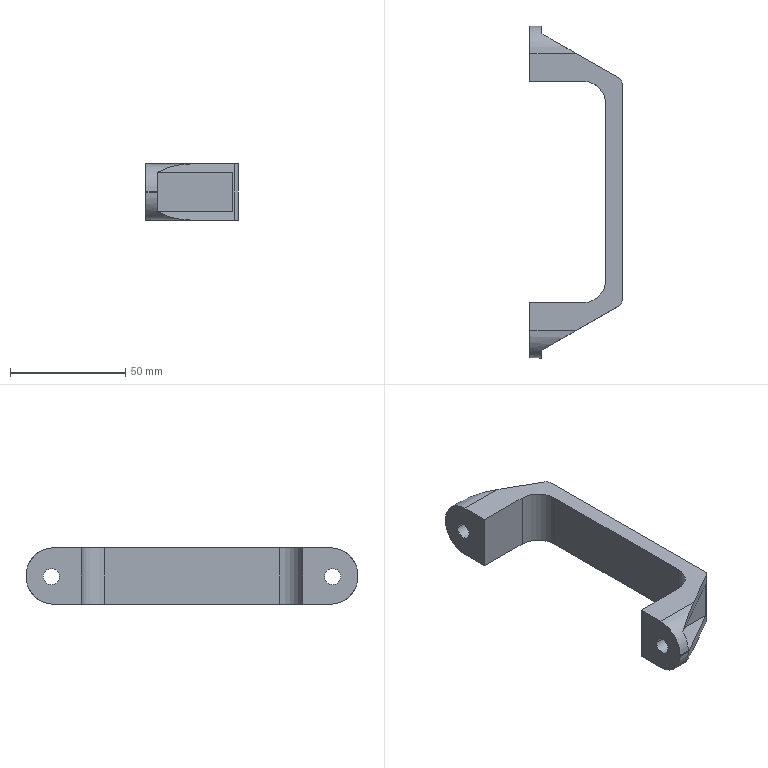Part | SolidWorks | features BaseBody 1 | 1 solid | 32 faces | box 40 x 144 x 24.5 mm | volume 30176 mm3 | plane 20 | cylinder 12 | commonest cylinder face diameters 7 x4 24 x4 6 x2 20 x2
STEP:
#1=CARTESIAN_POINT('',(-20.,-57.5,12.));
#2=VERTEX_POINT('',#1);
#3=CARTESIAN_POINT('',(-20.,-64.5,12.));
#4=VERTEX_POINT('',#3);
#5=CARTESIAN_POINT('',(-20.,-61.,12.));
#6=DIRECTION('',(-1.,0.,0.));
#7=DIRECTION('',(0.,1.,0.));
#8=AXIS2_PLACEMENT_3D('',#5,#6,#7);
#9=CIRCLE('',#8,3.5);
#10=EDGE_CURVE('',#2,#4,#9,.T.);
#11=ORIENTED_EDGE('',*,*,#10,.T.);
#12=CARTESIAN_POINT('',(-15.,-64.5,12.));
#13=VERTEX_POINT('',#12);
#14=CARTESIAN_POINT('',(-20.,-64.5,12.));
#15=DIRECTION('',(1.,0.,0.));
#16=VECTOR('',#15,1000.);
#17=LINE('',#14,#16);
#18=EDGE_CURVE('',#4,#13,#17,.T.);
#19=ORIENTED_EDGE('',*,*,#18,.T.);
#20=CARTESIAN_POINT('',(-15.,-57.5,12.));
#21=VERTEX_POINT('',#20);
#22=CARTESIAN_POINT('',(-15.,-61.,12.));
#23=DIRECTION('',(-1.,0.,0.));
#24=DIRECTION('',(0.,1.,0.));
#25=AXIS2_PLACEMENT_3D('',#22,#23,#24);
#26=CIRCLE('',#25,3.5);
#27=EDGE_CURVE('',#21,#13,#26,.T.);
#28=ORIENTED_EDGE('',*,*,#27,.F.);
#29=CARTESIAN_POINT('',(-20.,-57.5,12.));
#30=DIRECTION('',(1.,0.,0.));
#31=VECTOR('',#30,1000.);
#32=LINE('',#29,#31);
#33=EDGE_CURVE('',#2,#21,#32,.T.);
#34=ORIENTED_EDGE('',*,*,#33,.F.);
#35=EDGE_LOOP('',(#11,#19,#28,#34));
#36=FACE_OUTER_BOUND('',#35,.T.);
#37=CARTESIAN_POINT('',(-20.,-61.,12.));
#38=DIRECTION('',(1.,0.,0.));
#39=DIRECTION('',(0.,1.,0.));
#40=AXIS2_PLACEMENT_3D('',#37,#38,#39);
#41=CYLINDRICAL_SURFACE('',#40,3.5);
#42=ADVANCED_FACE('',(#36),#41,.F.);
#43=CARTESIAN_POINT('',(-20.,64.5,12.));
#44=VERTEX_POINT('',#43);
#45=CARTESIAN_POINT('',(-20.,57.5,12.));
#46=VERTEX_POINT('',#45);
#47=CARTESIAN_POINT('',(-20.,61.,12.));
#48=DIRECTION('',(-1.,0.,0.));
#49=DIRECTION('',(0.,1.,0.));
#50=AXIS2_PLACEMENT_3D('',#47,#48,#49);
#51=CIRCLE('',#50,3.5);
#52=EDGE_CURVE('',#44,#46,#51,.T.);
#53=ORIENTED_EDGE('',*,*,#52,.T.);
#54=CARTESIAN_POINT('',(-15.,57.5,12.));
#55=VERTEX_POINT('',#54);
#56=CARTESIAN_POINT('',(-20.,57.5,12.));
#57=DIRECTION('',(1.,0.,0.));
#58=VECTOR('',#57,1000.);
#59=LINE('',#56,#58);
#60=EDGE_CURVE('',#46,#55,#59,.T.);
#61=ORIENTED_EDGE('',*,*,#60,.T.);
#62=CARTESIAN_POINT('',(-15.,64.5,12.));
#63=VERTEX_POINT('',#62);
#64=CARTESIAN_POINT('',(-15.,61.,12.));
#65=DIRECTION('',(-1.,0.,0.));
#66=DIRECTION('',(0.,1.,0.));
#67=AXIS2_PLACEMENT_3D('',#64,#65,#66);
#68=CIRCLE('',#67,3.5);
#69=EDGE_CURVE('',#63,#55,#68,.T.);
#70=ORIENTED_EDGE('',*,*,#69,.F.);
#71=CARTESIAN_POINT('',(-20.,64.5,12.));
#72=DIRECTION('',(1.,0.,0.));
#73=VECTOR('',#72,1000.);
#74=LINE('',#71,#73);
#75=EDGE_CURVE('',#44,#63,#74,.T.);
#76=ORIENTED_EDGE('',*,*,#75,.F.);
#77=EDGE_LOOP('',(#53,#61,#70,#76));
#78=FACE_OUTER_BOUND('',#77,.T.);
#79=CARTESIAN_POINT('',(-20.,61.,12.));
#80=DIRECTION('',(1.,0.,0.));
#81=DIRECTION('',(0.,1.,0.));
#82=AXIS2_PLACEMENT_3D('',#79,#80,#81);
#83=CYLINDRICAL_SURFACE('',#82,3.5);
#84=ADVANCED_FACE('',(#78),#83,.F.);
#85=CARTESIAN_POINT('',(20.,-46.973,0.));
#86=VERTEX_POINT('',#85);
#87=CARTESIAN_POINT('',(20.,-46.973,24.5));
#88=VERTEX_POINT('',#87);
#89=CARTESIAN_POINT('',(20.,-46.973,24.5));
#90=DIRECTION('',(0.,0.,1.));
#91=VECTOR('',#90,1000.);
#92=LINE('',#89,#91);
#93=EDGE_CURVE('',#86,#88,#92,.T.);
#94=ORIENTED_EDGE('',*,*,#93,.F.);
#95=CARTESIAN_POINT('',(20.,46.973,0.));
#96=VERTEX_POINT('',#95);
#97=CARTESIAN_POINT('',(20.,72.,0.));
#98=DIRECTION('',(0.,-1.,0.));
#99=VECTOR('',#98,1000.);
#100=LINE('',#97,#99);
#101=EDGE_CURVE('',#96,#86,#100,.T.);
#102=ORIENTED_EDGE('',*,*,#101,.F.);
#103=CARTESIAN_POINT('',(20.,46.973,24.5));
#104=VERTEX_POINT('',#103);
#105=CARTESIAN_POINT('',(20.,46.973,24.5));
#106=DIRECTION('',(0.,0.,-1.));
#107=VECTOR('',#106,1000.);
#108=LINE('',#105,#107);
#109=EDGE_CURVE('',#104,#96,#108,.T.);
#110=ORIENTED_EDGE('',*,*,#109,.F.);
#111=CARTESIAN_POINT('',(20.,72.,24.5));
#112=DIRECTION('',(0.,1.,0.));
#113=VECTOR('',#112,1000.);
#114=LINE('',#111,#113);
#115=EDGE_CURVE('',#88,#104,#114,.T.);
#116=ORIENTED_EDGE('',*,*,#115,.F.);
#117=EDGE_LOOP('',(#94,#102,#110,#116));
#118=FACE_OUTER_BOUND('',#117,.T.);
#119=CARTESIAN_POINT('',(20.,72.,24.5));
#120=DIRECTION('',(-1.,0.,0.));
#121=DIRECTION('',(0.,-1.,0.));
#122=AXIS2_PLACEMENT_3D('',#119,#120,#121);
#123=PLANE('',#122);
#124=ADVANCED_FACE('',(#118),#123,.F.);
#125=CARTESIAN_POINT('',(-20.,-48.,24.5));
#126=VERTEX_POINT('',#125);
#127=CARTESIAN_POINT('',(-20.,-60.,24.5));
#128=VERTEX_POINT('',#127);
#129=CARTESIAN_POINT('',(-20.,0.,24.5));
#130=DIRECTION('',(0.,-1.,0.));
#131=VECTOR('',#130,1000.);
#132=LINE('',#129,#131);
#133=EDGE_CURVE('',#126,#128,#132,.T.);
#134=ORIENTED_EDGE('',*,*,#133,.T.);
#135=CARTESIAN_POINT('',(0.2499,-60.,24.5));
#136=VERTEX_POINT('',#135);
#137=CARTESIAN_POINT('',(0.,-60.,24.5));
#138=DIRECTION('',(1.,0.,0.));
#139=VECTOR('',#138,1000.);
#140=LINE('',#137,#139);
#141=EDGE_CURVE('',#128,#136,#140,.T.);
#142=ORIENTED_EDGE('',*,*,#141,.T.);
#143=CARTESIAN_POINT('',(18.488,-49.578,24.5));
#144=VERTEX_POINT('',#143);
#145=CARTESIAN_POINT('',(0.2499,-60.,24.5));
#146=DIRECTION('',(0.8682,0.4961,0.));
#147=VECTOR('',#146,1000.);
#148=LINE('',#145,#147);
#149=EDGE_CURVE('',#136,#144,#148,.T.);
#150=ORIENTED_EDGE('',*,*,#149,.T.);
#151=CARTESIAN_POINT('',(17.,-46.973,24.5));
#152=DIRECTION('',(0.,0.,1.));
#153=DIRECTION('',(1.,0.,0.));
#154=AXIS2_PLACEMENT_3D('',#151,#152,#153);
#155=CIRCLE('',#154,3.);
#156=EDGE_CURVE('',#144,#88,#155,.T.);
#157=ORIENTED_EDGE('',*,*,#156,.T.);
#158=ORIENTED_EDGE('',*,*,#115,.T.);
#159=CARTESIAN_POINT('',(18.488,49.578,24.5));
#160=VERTEX_POINT('',#159);
#161=CARTESIAN_POINT('',(17.,46.973,24.5));
#162=DIRECTION('',(0.,0.,1.));
#163=DIRECTION('',(1.,0.,0.));
#164=AXIS2_PLACEMENT_3D('',#161,#162,#163);
#165=CIRCLE('',#164,3.);
#166=EDGE_CURVE('',#104,#160,#165,.T.);
#167=ORIENTED_EDGE('',*,*,#166,.T.);
#168=CARTESIAN_POINT('',(0.2499,60.,24.5));
#169=VERTEX_POINT('',#168);
#170=CARTESIAN_POINT('',(18.488,49.578,24.5));
#171=DIRECTION('',(-0.8682,0.4961,0.));
#172=VECTOR('',#171,1000.);
#173=LINE('',#170,#172);
#174=EDGE_CURVE('',#160,#169,#173,.T.);
#175=ORIENTED_EDGE('',*,*,#174,.T.);
#176=CARTESIAN_POINT('',(-20.,60.,24.5));
#177=VERTEX_POINT('',#176);
#178=CARTESIAN_POINT('',(0.,60.,24.5));
#179=DIRECTION('',(-1.,0.,0.));
#180=VECTOR('',#179,1000.);
#181=LINE('',#178,#180);
#182=EDGE_CURVE('',#169,#177,#181,.T.);
#183=ORIENTED_EDGE('',*,*,#182,.T.);
#184=CARTESIAN_POINT('',(-20.,48.,24.5));
#185=VERTEX_POINT('',#184);
#186=CARTESIAN_POINT('',(-20.,0.,24.5));
#187=DIRECTION('',(0.,-1.,0.));
#188=VECTOR('',#187,1000.);
#189=LINE('',#186,#188);
#190=EDGE_CURVE('',#177,#185,#189,.T.);
#191=ORIENTED_EDGE('',*,*,#190,.T.);
#192=CARTESIAN_POINT('',(3.,48.,24.5));
#193=VERTEX_POINT('',#192);
#194=CARTESIAN_POINT('',(0.,48.,24.5));
#195=DIRECTION('',(1.,0.,0.));
#196=VECTOR('',#195,1000.);
#197=LINE('',#194,#196);
#198=EDGE_CURVE('',#185,#193,#197,.T.);
#199=ORIENTED_EDGE('',*,*,#198,.T.);
#200=CARTESIAN_POINT('',(13.,38.,24.5));
#201=VERTEX_POINT('',#200);
#202=CARTESIAN_POINT('',(3.,38.,24.5));
#203=DIRECTION('',(0.,0.,-1.));
#204=DIRECTION('',(1.,0.,0.));
#205=AXIS2_PLACEMENT_3D('',#202,#203,#204);
#206=CIRCLE('',#205,10.);
#207=EDGE_CURVE('',#193,#201,#206,.T.);
#208=ORIENTED_EDGE('',*,*,#207,.T.);
#209=CARTESIAN_POINT('',(13.,-38.,24.5));
#210=VERTEX_POINT('',#209);
#211=CARTESIAN_POINT('',(13.,0.,24.5));
#212=DIRECTION('',(0.,-1.,0.));
#213=VECTOR('',#212,1000.);
#214=LINE('',#211,#213);
#215=EDGE_CURVE('',#201,#210,#214,.T.);
#216=ORIENTED_EDGE('',*,*,#215,.T.);
#217=CARTESIAN_POINT('',(3.,-48.,24.5));
#218=VERTEX_POINT('',#217);
#219=CARTESIAN_POINT('',(3.,-38.,24.5));
#220=DIRECTION('',(0.,0.,-1.));
#221=DIRECTION('',(1.,0.,0.));
#222=AXIS2_PLACEMENT_3D('',#219,#220,#221);
#223=CIRCLE('',#222,10.);
#224=EDGE_CURVE('',#210,#218,#223,.T.);
#225=ORIENTED_EDGE('',*,*,#224,.T.);
#226=CARTESIAN_POINT('',(0.,-48.,24.5));
#227=DIRECTION('',(-1.,0.,0.));
#228=VECTOR('',#227,1000.);
#229=LINE('',#226,#228);
#230=EDGE_CURVE('',#218,#126,#229,.T.);
#231=ORIENTED_EDGE('',*,*,#230,.T.);
#232=EDGE_LOOP('',(#134,#142,#150,#157,#158,#167,#175,#183,#191,#199,#208,#216,#225,#231));
#233=FACE_OUTER_BOUND('',#232,.T.);
#234=CARTESIAN_POINT('',(0.,0.,24.5));
#235=DIRECTION('',(0.,0.,1.));
#236=DIRECTION('',(1.,0.,0.));
#237=AXIS2_PLACEMENT_3D('',#234,#235,#236);
#238=PLANE('',#237);
#239=ADVANCED_FACE('',(#233),#238,.T.);
#240=ORIENTED_EDGE('',*,*,#156,.F.);
#241=CARTESIAN_POINT('',(18.488,-49.578,0.));
#242=VERTEX_POINT('',#241);
#243=CARTESIAN_POINT('',(18.488,-49.578,0.));
#244=DIRECTION('',(0.,0.,-1.));
#245=VECTOR('',#244,1000.);
#246=LINE('',#243,#245);
#247=EDGE_CURVE('',#144,#242,#246,.T.);
#248=ORIENTED_EDGE('',*,*,#247,.T.);
#249=CARTESIAN_POINT('',(17.,-46.973,0.));
#250=DIRECTION('',(0.,0.,1.));
#251=DIRECTION('',(1.,0.,0.));
#252=AXIS2_PLACEMENT_3D('',#249,#250,#251);
#253=CIRCLE('',#252,3.);
#254=EDGE_CURVE('',#242,#86,#253,.T.);
#255=ORIENTED_EDGE('',*,*,#254,.T.);
#256=ORIENTED_EDGE('',*,*,#93,.T.);
#257=EDGE_LOOP('',(#240,#248,#255,#256));
#258=FACE_OUTER_BOUND('',#257,.T.);
#259=CARTESIAN_POINT('',(17.,-46.973,0.));
#260=DIRECTION('',(0.,0.,1.));
#261=DIRECTION('',(1.,0.,0.));
#262=AXIS2_PLACEMENT_3D('',#259,#260,#261);
#263=CYLINDRICAL_SURFACE('',#262,3.);
#264=ADVANCED_FACE('',(#258),#263,.T.);
#265=ORIENTED_EDGE('',*,*,#254,.F.);
#266=CARTESIAN_POINT('',(0.2499,-60.,0.));
#267=VERTEX_POINT('',#266);
#268=CARTESIAN_POINT('',(0.2499,-60.,0.));
#269=DIRECTION('',(0.8682,0.4961,0.));
#270=VECTOR('',#269,1000.);
#271=LINE('',#268,#270);
#272=EDGE_CURVE('',#267,#242,#271,.T.);
#273=ORIENTED_EDGE('',*,*,#272,.F.);
#274=CARTESIAN_POINT('',(-20.,-60.,0.));
#275=VERTEX_POINT('',#274);
#276=CARTESIAN_POINT('',(0.,-60.,0.));
#277=DIRECTION('',(1.,0.,0.));
#278=VECTOR('',#277,1000.);
#279=LINE('',#276,#278);
#280=EDGE_CURVE('',#275,#267,#279,.T.);
#281=ORIENTED_EDGE('',*,*,#280,.F.);
#282=CARTESIAN_POINT('',(-20.,-48.,0.));
#283=VERTEX_POINT('',#282);
#284=CARTESIAN_POINT('',(-20.,0.,0.));
#285=DIRECTION('',(0.,-1.,0.));
#286=VECTOR('',#285,1000.);
#287=LINE('',#284,#286);
#288=EDGE_CURVE('',#283,#275,#287,.T.);
#289=ORIENTED_EDGE('',*,*,#288,.F.);
#290=CARTESIAN_POINT('',(3.,-48.,0.));
#291=VERTEX_POINT('',#290);
#292=CARTESIAN_POINT('',(0.,-48.,0.));
#293=DIRECTION('',(-1.,0.,0.));
#294=VECTOR('',#293,1000.);
#295=LINE('',#292,#294);
#296=EDGE_CURVE('',#291,#283,#295,.T.);
#297=ORIENTED_EDGE('',*,*,#296,.F.);
#298=CARTESIAN_POINT('',(13.,-38.,0.));
#299=VERTEX_POINT('',#298);
#300=CARTESIAN_POINT('',(3.,-38.,0.));
#301=DIRECTION('',(0.,0.,-1.));
#302=DIRECTION('',(1.,0.,0.));
#303=AXIS2_PLACEMENT_3D('',#300,#301,#302);
#304=CIRCLE('',#303,10.);
#305=EDGE_CURVE('',#299,#291,#304,.T.);
#306=ORIENTED_EDGE('',*,*,#305,.F.);
#307=CARTESIAN_POINT('',(13.,38.,0.));
#308=VERTEX_POINT('',#307);
#309=CARTESIAN_POINT('',(13.,0.,0.));
#310=DIRECTION('',(0.,-1.,0.));
#311=VECTOR('',#310,1000.);
#312=LINE('',#309,#311);
#313=EDGE_CURVE('',#308,#299,#312,.T.);
#314=ORIENTED_EDGE('',*,*,#313,.F.);
#315=CARTESIAN_POINT('',(3.,48.,0.));
#316=VERTEX_POINT('',#315);
#317=CARTESIAN_POINT('',(3.,38.,0.));
#318=DIRECTION('',(0.,0.,-1.));
#319=DIRECTION('',(1.,0.,0.));
#320=AXIS2_PLACEMENT_3D('',#317,#318,#319);
#321=CIRCLE('',#320,10.);
#322=EDGE_CURVE('',#316,#308,#321,.T.);
#323=ORIENTED_EDGE('',*,*,#322,.F.);
#324=CARTESIAN_POINT('',(-20.,48.,0.));
#325=VERTEX_POINT('',#324);
#326=CARTESIAN_POINT('',(0.,48.,0.));
#327=DIRECTION('',(1.,0.,0.));
#328=VECTOR('',#327,1000.);
#329=LINE('',#326,#328);
#330=EDGE_CURVE('',#325,#316,#329,.T.);
#331=ORIENTED_EDGE('',*,*,#330,.F.);
#332=CARTESIAN_POINT('',(-20.,60.,0.));
#333=VERTEX_POINT('',#332);
#334=CARTESIAN_POINT('',(-20.,0.,0.));
#335=DIRECTION('',(0.,-1.,0.));
#336=VECTOR('',#335,1000.);
#337=LINE('',#334,#336);
#338=EDGE_CURVE('',#333,#325,#337,.T.);
#339=ORIENTED_EDGE('',*,*,#338,.F.);
#340=CARTESIAN_POINT('',(0.2499,60.,0.));
#341=VERTEX_POINT('',#340);
#342=CARTESIAN_POINT('',(0.,60.,0.));
#343=DIRECTION('',(-1.,0.,0.));
#344=VECTOR('',#343,1000.);
#345=LINE('',#342,#344);
#346=EDGE_CURVE('',#341,#333,#345,.T.);
#347=ORIENTED_EDGE('',*,*,#346,.F.);
#348=CARTESIAN_POINT('',(18.488,49.578,0.));
#349=VERTEX_POINT('',#348);
#350=CARTESIAN_POINT('',(18.488,49.578,0.));
#351=DIRECTION('',(-0.8682,0.4961,0.));
#352=VECTOR('',#351,1000.);
#353=LINE('',#350,#352);
#354=EDGE_CURVE('',#349,#341,#353,.T.);
#355=ORIENTED_EDGE('',*,*,#354,.F.);
#356=CARTESIAN_POINT('',(17.,46.973,0.));
#357=DIRECTION('',(0.,0.,1.));
#358=DIRECTION('',(1.,0.,0.));
#359=AXIS2_PLACEMENT_3D('',#356,#357,#358);
#360=CIRCLE('',#359,3.);
#361=EDGE_CURVE('',#96,#349,#360,.T.);
#362=ORIENTED_EDGE('',*,*,#361,.F.);
#363=ORIENTED_EDGE('',*,*,#101,.T.);
#364=EDGE_LOOP('',(#265,#273,#281,#289,#297,#306,#314,#323,#331,#339,#347,#355,#362,#363));
#365=FACE_OUTER_BOUND('',#364,.T.);
#366=CARTESIAN_POINT('',(0.,0.,0.));
#367=DIRECTION('',(0.,0.,1.));
#368=DIRECTION('',(1.,0.,0.));
#369=AXIS2_PLACEMENT_3D('',#366,#367,#368);
#370=PLANE('',#369);
#371=ADVANCED_FACE('',(#365),#370,.F.);
#372=ORIENTED_EDGE('',*,*,#166,.F.);
#373=ORIENTED_EDGE('',*,*,#109,.T.);
#374=ORIENTED_EDGE('',*,*,#361,.T.);
#375=CARTESIAN_POINT('',(18.488,49.578,24.5));
#376=DIRECTION('',(0.,0.,1.));
#377=VECTOR('',#376,1000.);
#378=LINE('',#375,#377);
#379=EDGE_CURVE('',#349,#160,#378,.T.);
#380=ORIENTED_EDGE('',*,*,#379,.T.);
#381=EDGE_LOOP('',(#372,#373,#374,#380));
#382=FACE_OUTER_BOUND('',#381,.T.);
#383=CARTESIAN_POINT('',(17.,46.973,24.5));
#384=DIRECTION('',(0.,0.,1.));
#385=DIRECTION('',(1.,0.,0.));
#386=AXIS2_PLACEMENT_3D('',#383,#384,#385);
#387=CYLINDRICAL_SURFACE('',#386,3.);
#388=ADVANCED_FACE('',(#382),#387,.T.);
#389=CARTESIAN_POINT('',(-20.,-72.,12.5));
#390=VERTEX_POINT('',#389);
#391=CARTESIAN_POINT('',(-15.,-72.,12.5));
#392=VERTEX_POINT('',#391);
#393=CARTESIAN_POINT('',(0.,-72.,12.5));
#394=DIRECTION('',(1.,0.,0.));
#395=VECTOR('',#394,1000.);
#396=LINE('',#393,#395);
#397=EDGE_CURVE('',#390,#392,#396,.T.);
#398=ORIENTED_EDGE('',*,*,#397,.T.);
#399=CARTESIAN_POINT('',(-15.,-68.714,20.75));
#400=VERTEX_POINT('',#399);
#401=CARTESIAN_POINT('',(-15.,-60.,12.5));
#402=DIRECTION('',(-1.,0.,0.));
#403=DIRECTION('',(0.,0.,1.));
#404=AXIS2_PLACEMENT_3D('',#401,#402,#403);
#405=CIRCLE('',#404,12.);
#406=EDGE_CURVE('',#392,#400,#405,.T.);
#407=ORIENTED_EDGE('',*,*,#406,.T.);
#408=CARTESIAN_POINT('',(-15.,-68.714,20.75));
#409=CARTESIAN_POINT('',(-10.977,-66.415,23.178));
#410=CARTESIAN_POINT('',(-5.602,-63.344,24.5));
#411=CARTESIAN_POINT('',(0.2499,-60.,24.5));
#412=(BOUNDED_CURVE()B_SPLINE_CURVE(3,(#408,#409,#410,#411),.UNSPECIFIED.,.F.,.F.)B_SPLINE_CURVE_WITH_KNOTS((4,4),(0.758,1.571),.UNSPECIFIED.)CURVE()GEOMETRIC_REPRESENTATION_ITEM()RATIONAL_B_SPLINE_CURVE((1.,0.9457,0.9457,1.))REPRESENTATION_ITEM(''));
#413=EDGE_CURVE('',#400,#136,#412,.T.);
#414=ORIENTED_EDGE('',*,*,#413,.T.);
#415=ORIENTED_EDGE('',*,*,#141,.F.);
#416=CARTESIAN_POINT('',(-20.,-60.,12.5));
#417=DIRECTION('',(1.,0.,0.));
#418=DIRECTION('',(0.,0.,1.));
#419=AXIS2_PLACEMENT_3D('',#416,#417,#418);
#420=CIRCLE('',#419,12.);
#421=EDGE_CURVE('',#128,#390,#420,.T.);
#422=ORIENTED_EDGE('',*,*,#421,.T.);
#423=EDGE_LOOP('',(#398,#407,#414,#415,#422));
#424=FACE_OUTER_BOUND('',#423,.T.);
#425=CARTESIAN_POINT('',(0.,-60.,12.5));
#426=DIRECTION('',(-1.,0.,0.));
#427=DIRECTION('',(0.,0.,1.));
#428=AXIS2_PLACEMENT_3D('',#425,#426,#427);
#429=CYLINDRICAL_SURFACE('',#428,12.);
#430=ADVANCED_FACE('',(#424),#429,.T.);
#431=ORIENTED_EDGE('',*,*,#421,.F.);
#432=ORIENTED_EDGE('',*,*,#133,.F.);
#433=CARTESIAN_POINT('',(-20.,-48.,24.5));
#434=DIRECTION('',(0.,0.,1.));
#435=VECTOR('',#434,1000.);
#436=LINE('',#433,#435);
#437=EDGE_CURVE('',#283,#126,#436,.T.);
#438=ORIENTED_EDGE('',*,*,#437,.F.);
#439=ORIENTED_EDGE('',*,*,#288,.T.);
#440=CARTESIAN_POINT('',(-20.,-72.,12.));
#441=VERTEX_POINT('',#440);
#442=CARTESIAN_POINT('',(-20.,-60.,12.));
#443=DIRECTION('',(1.,0.,0.));
#444=DIRECTION('',(0.,0.,-1.));
#445=AXIS2_PLACEMENT_3D('',#442,#443,#444);
#446=CIRCLE('',#445,12.);
#447=EDGE_CURVE('',#441,#275,#446,.T.);
#448=ORIENTED_EDGE('',*,*,#447,.F.);
#449=CARTESIAN_POINT('',(-20.,-72.,24.5));
#450=DIRECTION('',(0.,0.,-1.));
#451=VECTOR('',#450,1000.);
#452=LINE('',#449,#451);
#453=EDGE_CURVE('',#390,#441,#452,.T.);
#454=ORIENTED_EDGE('',*,*,#453,.F.);
#455=EDGE_LOOP('',(#431,#432,#438,#439,#448,#454));
#456=FACE_OUTER_BOUND('',#455,.T.);
#457=ORIENTED_EDGE('',*,*,#10,.F.);
#458=CARTESIAN_POINT('',(-20.,-61.,12.));
#459=DIRECTION('',(-1.,0.,0.));
#460=DIRECTION('',(0.,1.,0.));
#461=AXIS2_PLACEMENT_3D('',#458,#459,#460);
#462=CIRCLE('',#461,3.5);
#463=EDGE_CURVE('',#4,#2,#462,.T.);
#464=ORIENTED_EDGE('',*,*,#463,.F.);
#465=EDGE_LOOP('',(#457,#464));
#466=FACE_BOUND('',#465,.T.);
#467=CARTESIAN_POINT('',(-20.,72.,24.5));
#468=DIRECTION('',(1.,0.,0.));
#469=DIRECTION('',(0.,1.,0.));
#470=AXIS2_PLACEMENT_3D('',#467,#468,#469);
#471=PLANE('',#470);
#472=ADVANCED_FACE('',(#456,#466),#471,.F.);
#473=ORIENTED_EDGE('',*,*,#296,.T.);
#474=ORIENTED_EDGE('',*,*,#437,.T.);
#475=ORIENTED_EDGE('',*,*,#230,.F.);
#476=CARTESIAN_POINT('',(3.,-48.,0.));
#477=DIRECTION('',(0.,0.,-1.));
#478=VECTOR('',#477,1000.);
#479=LINE('',#476,#478);
#480=EDGE_CURVE('',#218,#291,#479,.T.);
#481=ORIENTED_EDGE('',*,*,#480,.T.);
#482=EDGE_LOOP('',(#473,#474,#475,#481));
#483=FACE_OUTER_BOUND('',#482,.T.);
#484=CARTESIAN_POINT('',(3.,-48.,0.));
#485=DIRECTION('',(0.,1.,0.));
#486=DIRECTION('',(-1.,0.,0.));
#487=AXIS2_PLACEMENT_3D('',#484,#485,#486);
#488=PLANE('',#487);
#489=ADVANCED_FACE('',(#483),#488,.T.);
#490=CARTESIAN_POINT('',(13.,-38.,0.));
#491=DIRECTION('',(0.,0.,1.));
#492=VECTOR('',#491,1000.);
#493=LINE('',#490,#492);
#494=EDGE_CURVE('',#299,#210,#493,.T.);
#495=ORIENTED_EDGE('',*,*,#494,.F.);
#496=ORIENTED_EDGE('',*,*,#305,.T.);
#497=ORIENTED_EDGE('',*,*,#480,.F.);
#498=ORIENTED_EDGE('',*,*,#224,.F.);
#499=EDGE_LOOP('',(#495,#496,#497,#498));
#500=FACE_OUTER_BOUND('',#499,.T.);
#501=CARTESIAN_POINT('',(3.,-38.,0.));
#502=DIRECTION('',(0.,0.,1.));
#503=DIRECTION('',(1.,0.,0.));
#504=AXIS2_PLACEMENT_3D('',#501,#502,#503);
#505=CYLINDRICAL_SURFACE('',#504,10.);
#506=ADVANCED_FACE('',(#500),#505,.F.);
#507=CARTESIAN_POINT('',(13.,38.,0.));
#508=DIRECTION('',(0.,0.,1.));
#509=VECTOR('',#508,1000.);
#510=LINE('',#507,#509);
#511=EDGE_CURVE('',#308,#201,#510,.T.);
#512=ORIENTED_EDGE('',*,*,#511,.F.);
#513=ORIENTED_EDGE('',*,*,#313,.T.);
#514=ORIENTED_EDGE('',*,*,#494,.T.);
#515=ORIENTED_EDGE('',*,*,#215,.F.);
#516=EDGE_LOOP('',(#512,#513,#514,#515));
#517=FACE_OUTER_BOUND('',#516,.T.);
#518=CARTESIAN_POINT('',(13.,-38.,0.));
#519=DIRECTION('',(1.,0.,0.));
#520=DIRECTION('',(0.,0.,-1.));
#521=AXIS2_PLACEMENT_3D('',#518,#519,#520);
#522=PLANE('',#521);
#523=ADVANCED_FACE('',(#517),#522,.F.);
#524=CARTESIAN_POINT('',(3.,48.,0.));
#525=DIRECTION('',(0.,0.,1.));
#526=VECTOR('',#525,1000.);
#527=LINE('',#524,#526);
#528=EDGE_CURVE('',#316,#193,#527,.T.);
#529=ORIENTED_EDGE('',*,*,#528,.F.);
#530=ORIENTED_EDGE('',*,*,#322,.T.);
#531=ORIENTED_EDGE('',*,*,#511,.T.);
#532=ORIENTED_EDGE('',*,*,#207,.F.);
#533=EDGE_LOOP('',(#529,#530,#531,#532));
#534=FACE_OUTER_BOUND('',#533,.T.);
#535=CARTESIAN_POINT('',(3.,38.,0.));
#536=DIRECTION('',(0.,0.,1.));
#537=DIRECTION('',(1.,0.,0.));
#538=AXIS2_PLACEMENT_3D('',#535,#536,#537);
#539=CYLINDRICAL_SURFACE('',#538,10.);
#540=ADVANCED_FACE('',(#534),#539,.F.);
#541=CARTESIAN_POINT('',(-20.,48.,0.));
#542=DIRECTION('',(0.,0.,1.));
#543=VECTOR('',#542,1000.);
#544=LINE('',#541,#543);
#545=EDGE_CURVE('',#325,#185,#544,.T.);
#546=ORIENTED_EDGE('',*,*,#545,.F.);
#547=ORIENTED_EDGE('',*,*,#330,.T.);
#548=ORIENTED_EDGE('',*,*,#528,.T.);
#549=ORIENTED_EDGE('',*,*,#198,.F.);
#550=EDGE_LOOP('',(#546,#547,#548,#549));
#551=FACE_OUTER_BOUND('',#550,.T.);
#552=CARTESIAN_POINT('',(3.,48.,0.));
#553=DIRECTION('',(0.,1.,0.));
#554=DIRECTION('',(-1.,0.,0.));
#555=AXIS2_PLACEMENT_3D('',#552,#553,#554);
#556=PLANE('',#555);
#557=ADVANCED_FACE('',(#551),#556,.F.);
#558=CARTESIAN_POINT('',(-20.,72.,12.));
#559=VERTEX_POINT('',#558);
#560=CARTESIAN_POINT('',(-20.,60.,12.));
#561=DIRECTION('',(1.,0.,0.));
#562=DIRECTION('',(0.,0.,1.));
#563=AXIS2_PLACEMENT_3D('',#560,#561,#562);
#564=CIRCLE('',#563,12.);
#565=EDGE_CURVE('',#333,#559,#564,.T.);
#566=ORIENTED_EDGE('',*,*,#565,.F.);
#567=ORIENTED_EDGE('',*,*,#338,.T.);
#568=ORIENTED_EDGE('',*,*,#545,.T.);
#569=ORIENTED_EDGE('',*,*,#190,.F.);
#570=CARTESIAN_POINT('',(-20.,72.,12.5));
#571=VERTEX_POINT('',#570);
#572=CARTESIAN_POINT('',(-20.,60.,12.5));
#573=DIRECTION('',(1.,0.,0.));
#574=DIRECTION('',(0.,0.,-1.));
#575=AXIS2_PLACEMENT_3D('',#572,#573,#574);
#576=CIRCLE('',#575,12.);
#577=EDGE_CURVE('',#571,#177,#576,.T.);
#578=ORIENTED_EDGE('',*,*,#577,.F.);
#579=CARTESIAN_POINT('',(-20.,72.,24.5));
#580=DIRECTION('',(0.,0.,-1.));
#581=VECTOR('',#580,1000.);
#582=LINE('',#579,#581);
#583=EDGE_CURVE('',#571,#559,#582,.T.);
#584=ORIENTED_EDGE('',*,*,#583,.T.);
#585=EDGE_LOOP('',(#566,#567,#568,#569,#578,#584));
#586=FACE_OUTER_BOUND('',#585,.T.);
#587=ORIENTED_EDGE('',*,*,#52,.F.);
#588=CARTESIAN_POINT('',(-20.,61.,12.));
#589=DIRECTION('',(-1.,0.,0.));
#590=DIRECTION('',(0.,1.,0.));
#591=AXIS2_PLACEMENT_3D('',#588,#589,#590);
#592=CIRCLE('',#591,3.5);
#593=EDGE_CURVE('',#46,#44,#592,.T.);
#594=ORIENTED_EDGE('',*,*,#593,.F.);
#595=EDGE_LOOP('',(#587,#594));
#596=FACE_BOUND('',#595,.T.);
#597=CARTESIAN_POINT('',(-20.,72.,24.5));
#598=DIRECTION('',(1.,0.,0.));
#599=DIRECTION('',(0.,1.,0.));
#600=AXIS2_PLACEMENT_3D('',#597,#598,#599);
#601=PLANE('',#600);
#602=ADVANCED_FACE('',(#586,#596),#601,.F.);
#603=ORIENTED_EDGE('',*,*,#577,.T.);
#604=ORIENTED_EDGE('',*,*,#182,.F.);
#605=CARTESIAN_POINT('',(-15.,68.714,20.75));
#606=VERTEX_POINT('',#605);
#607=CARTESIAN_POINT('',(0.2499,60.,24.5));
#608=CARTESIAN_POINT('',(-5.602,63.344,24.5));
#609=CARTESIAN_POINT('',(-10.977,66.415,23.178));
#610=CARTESIAN_POINT('',(-15.,68.714,20.75));
#611=(BOUNDED_CURVE()B_SPLINE_CURVE(3,(#607,#608,#609,#610),.UNSPECIFIED.,.F.,.F.)B_SPLINE_CURVE_WITH_KNOTS((4,4),(1.571,2.384),.UNSPECIFIED.)CURVE()GEOMETRIC_REPRESENTATION_ITEM()RATIONAL_B_SPLINE_CURVE((1.,0.9457,0.9457,1.))REPRESENTATION_ITEM(''));
#612=EDGE_CURVE('',#169,#606,#611,.T.);
#613=ORIENTED_EDGE('',*,*,#612,.T.);
#614=CARTESIAN_POINT('',(-15.,72.,12.5));
#615=VERTEX_POINT('',#614);
#616=CARTESIAN_POINT('',(-15.,60.,12.5));
#617=DIRECTION('',(-1.,0.,0.));
#618=DIRECTION('',(0.,0.,-1.));
#619=AXIS2_PLACEMENT_3D('',#616,#617,#618);
#620=CIRCLE('',#619,12.);
#621=EDGE_CURVE('',#606,#615,#620,.T.);
#622=ORIENTED_EDGE('',*,*,#621,.T.);
#623=CARTESIAN_POINT('',(0.,72.,12.5));
#624=DIRECTION('',(-1.,0.,0.));
#625=VECTOR('',#624,1000.);
#626=LINE('',#623,#625);
#627=EDGE_CURVE('',#615,#571,#626,.T.);
#628=ORIENTED_EDGE('',*,*,#627,.T.);
#629=EDGE_LOOP('',(#603,#604,#613,#622,#628));
#630=FACE_OUTER_BOUND('',#629,.T.);
#631=CARTESIAN_POINT('',(0.,60.,12.5));
#632=DIRECTION('',(1.,0.,0.));
#633=DIRECTION('',(0.,0.,-1.));
#634=AXIS2_PLACEMENT_3D('',#631,#632,#633);
#635=CYLINDRICAL_SURFACE('',#634,12.);
#636=ADVANCED_FACE('',(#630),#635,.T.);
#637=ORIENTED_EDGE('',*,*,#379,.F.);
#638=ORIENTED_EDGE('',*,*,#354,.T.);
#639=CARTESIAN_POINT('',(-15.,68.714,3.75));
#640=VERTEX_POINT('',#639);
#641=CARTESIAN_POINT('',(-15.,68.714,3.75));
#642=CARTESIAN_POINT('',(-10.977,66.415,1.322));
#643=CARTESIAN_POINT('',(-5.602,63.344,0.));
#644=CARTESIAN_POINT('',(0.2499,60.,0.));
#645=(BOUNDED_CURVE()B_SPLINE_CURVE(3,(#641,#642,#643,#644),.UNSPECIFIED.,.F.,.F.)B_SPLINE_CURVE_WITH_KNOTS((4,4),(0.758,1.571),.UNSPECIFIED.)CURVE()GEOMETRIC_REPRESENTATION_ITEM()RATIONAL_B_SPLINE_CURVE((1.,0.9457,0.9457,1.))REPRESENTATION_ITEM(''));
#646=EDGE_CURVE('',#640,#341,#645,.T.);
#647=ORIENTED_EDGE('',*,*,#646,.F.);
#648=CARTESIAN_POINT('',(17.75,50.,3.75));
#649=VERTEX_POINT('',#648);
#650=CARTESIAN_POINT('',(-15.,68.714,3.75));
#651=DIRECTION('',(-0.8682,0.4961,0.));
#652=VECTOR('',#651,1000.);
#653=LINE('',#650,#652);
#654=EDGE_CURVE('',#649,#640,#653,.T.);
#655=ORIENTED_EDGE('',*,*,#654,.F.);
#656=CARTESIAN_POINT('',(17.75,50.,20.75));
#657=VERTEX_POINT('',#656);
#658=CARTESIAN_POINT('',(17.75,50.,0.));
#659=DIRECTION('',(0.,0.,-1.));
#660=VECTOR('',#659,1000.);
#661=LINE('',#658,#660);
#662=EDGE_CURVE('',#657,#649,#661,.T.);
#663=ORIENTED_EDGE('',*,*,#662,.F.);
#664=CARTESIAN_POINT('',(-15.,68.714,20.75));
#665=DIRECTION('',(0.8682,-0.4961,0.));
#666=VECTOR('',#665,1000.);
#667=LINE('',#664,#666);
#668=EDGE_CURVE('',#606,#657,#667,.T.);
#669=ORIENTED_EDGE('',*,*,#668,.F.);
#670=ORIENTED_EDGE('',*,*,#612,.F.);
#671=ORIENTED_EDGE('',*,*,#174,.F.);
#672=EDGE_LOOP('',(#637,#638,#647,#655,#663,#669,#670,#671));
#673=FACE_OUTER_BOUND('',#672,.T.);
#674=CARTESIAN_POINT('',(-15.,68.714,0.));
#675=DIRECTION('',(-0.4961,-0.8682,0.));
#676=DIRECTION('',(0.8682,-0.4961,0.));
#677=AXIS2_PLACEMENT_3D('',#674,#675,#676);
#678=PLANE('',#677);
#679=ADVANCED_FACE('',(#673),#678,.F.);
#680=ORIENTED_EDGE('',*,*,#247,.F.);
#681=ORIENTED_EDGE('',*,*,#149,.F.);
#682=ORIENTED_EDGE('',*,*,#413,.F.);
#683=CARTESIAN_POINT('',(17.75,-50.,20.75));
#684=VERTEX_POINT('',#683);
#685=CARTESIAN_POINT('',(-15.,-68.714,20.75));
#686=DIRECTION('',(-0.8682,-0.4961,0.));
#687=VECTOR('',#686,1000.);
#688=LINE('',#685,#687);
#689=EDGE_CURVE('',#684,#400,#688,.T.);
#690=ORIENTED_EDGE('',*,*,#689,.F.);
#691=CARTESIAN_POINT('',(17.75,-50.,3.75));
#692=VERTEX_POINT('',#691);
#693=CARTESIAN_POINT('',(17.75,-50.,0.));
#694=DIRECTION('',(0.,0.,1.));
#695=VECTOR('',#694,1000.);
#696=LINE('',#693,#695);
#697=EDGE_CURVE('',#692,#684,#696,.T.);
#698=ORIENTED_EDGE('',*,*,#697,.F.);
#699=CARTESIAN_POINT('',(-15.,-68.714,3.75));
#700=VERTEX_POINT('',#699);
#701=CARTESIAN_POINT('',(-15.,-68.714,3.75));
#702=DIRECTION('',(0.8682,0.4961,0.));
#703=VECTOR('',#702,1000.);
#704=LINE('',#701,#703);
#705=EDGE_CURVE('',#700,#692,#704,.T.);
#706=ORIENTED_EDGE('',*,*,#705,.F.);
#707=CARTESIAN_POINT('',(0.2499,-60.,0.));
#708=CARTESIAN_POINT('',(-5.602,-63.344,0.));
#709=CARTESIAN_POINT('',(-10.977,-66.415,1.322));
#710=CARTESIAN_POINT('',(-15.,-68.714,3.75));
#711=(BOUNDED_CURVE()B_SPLINE_CURVE(3,(#707,#708,#709,#710),.UNSPECIFIED.,.F.,.F.)B_SPLINE_CURVE_WITH_KNOTS((4,4),(1.571,2.384),.UNSPECIFIED.)CURVE()GEOMETRIC_REPRESENTATION_ITEM()RATIONAL_B_SPLINE_CURVE((1.,0.9457,0.9457,1.))REPRESENTATION_ITEM(''));
#712=EDGE_CURVE('',#267,#700,#711,.T.);
#713=ORIENTED_EDGE('',*,*,#712,.F.);
#714=ORIENTED_EDGE('',*,*,#272,.T.);
#715=EDGE_LOOP('',(#680,#681,#682,#690,#698,#706,#713,#714));
#716=FACE_OUTER_BOUND('',#715,.T.);
#717=CARTESIAN_POINT('',(-15.,-68.714,0.));
#718=DIRECTION('',(-0.4961,0.8682,0.));
#719=DIRECTION('',(-0.8682,-0.4961,0.));
#720=AXIS2_PLACEMENT_3D('',#717,#718,#719);
#721=PLANE('',#720);
#722=ADVANCED_FACE('',(#716),#721,.F.);
#723=ORIENTED_EDGE('',*,*,#447,.T.);
#724=ORIENTED_EDGE('',*,*,#280,.T.);
#725=ORIENTED_EDGE('',*,*,#712,.T.);
#726=CARTESIAN_POINT('',(-15.,-72.,12.));
#727=VERTEX_POINT('',#726);
#728=CARTESIAN_POINT('',(-15.,-60.,12.));
#729=DIRECTION('',(-1.,0.,0.));
#730=DIRECTION('',(0.,0.,-1.));
#731=AXIS2_PLACEMENT_3D('',#728,#729,#730);
#732=CIRCLE('',#731,12.);
#733=EDGE_CURVE('',#700,#727,#732,.T.);
#734=ORIENTED_EDGE('',*,*,#733,.T.);
#735=CARTESIAN_POINT('',(-20.,-72.,12.));
#736=DIRECTION('',(-1.,0.,0.));
#737=VECTOR('',#736,1000.);
#738=LINE('',#735,#737);
#739=EDGE_CURVE('',#727,#441,#738,.T.);
#740=ORIENTED_EDGE('',*,*,#739,.T.);
#741=EDGE_LOOP('',(#723,#724,#725,#734,#740));
#742=FACE_OUTER_BOUND('',#741,.T.);
#743=CARTESIAN_POINT('',(-20.,-60.,12.));
#744=DIRECTION('',(1.,0.,0.));
#745=DIRECTION('',(0.,0.,-1.));
#746=AXIS2_PLACEMENT_3D('',#743,#744,#745);
#747=CYLINDRICAL_SURFACE('',#746,12.);
#748=ADVANCED_FACE('',(#742),#747,.T.);
#749=CARTESIAN_POINT('',(-15.,72.,12.));
#750=VERTEX_POINT('',#749);
#751=CARTESIAN_POINT('',(-20.,72.,12.));
#752=DIRECTION('',(1.,0.,0.));
#753=VECTOR('',#752,1000.);
#754=LINE('',#751,#753);
#755=EDGE_CURVE('',#559,#750,#754,.T.);
#756=ORIENTED_EDGE('',*,*,#755,.T.);
#757=CARTESIAN_POINT('',(-15.,60.,12.));
#758=DIRECTION('',(-1.,0.,0.));
#759=DIRECTION('',(0.,0.,1.));
#760=AXIS2_PLACEMENT_3D('',#757,#758,#759);
#761=CIRCLE('',#760,12.);
#762=EDGE_CURVE('',#750,#640,#761,.T.);
#763=ORIENTED_EDGE('',*,*,#762,.T.);
#764=ORIENTED_EDGE('',*,*,#646,.T.);
#765=ORIENTED_EDGE('',*,*,#346,.T.);
#766=ORIENTED_EDGE('',*,*,#565,.T.);
#767=EDGE_LOOP('',(#756,#763,#764,#765,#766));
#768=FACE_OUTER_BOUND('',#767,.T.);
#769=CARTESIAN_POINT('',(-20.,60.,12.));
#770=DIRECTION('',(-1.,0.,0.));
#771=DIRECTION('',(0.,0.,1.));
#772=AXIS2_PLACEMENT_3D('',#769,#770,#771);
#773=CYLINDRICAL_SURFACE('',#772,12.);
#774=ADVANCED_FACE('',(#768),#773,.T.);
#775=CARTESIAN_POINT('',(-15.,-50.,3.75));
#776=VERTEX_POINT('',#775);
#777=CARTESIAN_POINT('',(-15.,72.,3.75));
#778=DIRECTION('',(0.,1.,0.));
#779=VECTOR('',#778,1000.);
#780=LINE('',#777,#779);
#781=EDGE_CURVE('',#700,#776,#780,.T.);
#782=ORIENTED_EDGE('',*,*,#781,.T.);
#783=CARTESIAN_POINT('',(-15.,-50.,20.75));
#784=VERTEX_POINT('',#783);
#785=CARTESIAN_POINT('',(-15.,-50.,24.5));
#786=DIRECTION('',(0.,0.,1.));
#787=VECTOR('',#786,1000.);
#788=LINE('',#785,#787);
#789=EDGE_CURVE('',#776,#784,#788,.T.);
#790=ORIENTED_EDGE('',*,*,#789,.T.);
#791=CARTESIAN_POINT('',(-15.,72.,20.75));
#792=DIRECTION('',(0.,-1.,0.));
#793=VECTOR('',#792,1000.);
#794=LINE('',#791,#793);
#795=EDGE_CURVE('',#784,#400,#794,.T.);
#796=ORIENTED_EDGE('',*,*,#795,.T.);
#797=ORIENTED_EDGE('',*,*,#406,.F.);
#798=CARTESIAN_POINT('',(-15.,-72.,24.5));
#799=DIRECTION('',(0.,0.,-1.));
#800=VECTOR('',#799,1000.);
#801=LINE('',#798,#800);
#802=EDGE_CURVE('',#392,#727,#801,.T.);
#803=ORIENTED_EDGE('',*,*,#802,.T.);
#804=ORIENTED_EDGE('',*,*,#733,.F.);
#805=EDGE_LOOP('',(#782,#790,#796,#797,#803,#804));
#806=FACE_OUTER_BOUND('',#805,.T.);
#807=ORIENTED_EDGE('',*,*,#27,.T.);
#808=CARTESIAN_POINT('',(-15.,-61.,12.));
#809=DIRECTION('',(-1.,0.,0.));
#810=DIRECTION('',(0.,1.,0.));
#811=AXIS2_PLACEMENT_3D('',#808,#809,#810);
#812=CIRCLE('',#811,3.5);
#813=EDGE_CURVE('',#13,#21,#812,.T.);
#814=ORIENTED_EDGE('',*,*,#813,.T.);
#815=EDGE_LOOP('',(#807,#814));
#816=FACE_BOUND('',#815,.T.);
#817=CARTESIAN_POINT('',(-15.,72.,24.5));
#818=DIRECTION('',(1.,0.,0.));
#819=DIRECTION('',(0.,1.,0.));
#820=AXIS2_PLACEMENT_3D('',#817,#818,#819);
#821=PLANE('',#820);
#822=ADVANCED_FACE('',(#806,#816),#821,.T.);
#823=ORIENTED_EDGE('',*,*,#397,.F.);
#824=ORIENTED_EDGE('',*,*,#453,.T.);
#825=ORIENTED_EDGE('',*,*,#739,.F.);
#826=ORIENTED_EDGE('',*,*,#802,.F.);
#827=EDGE_LOOP('',(#823,#824,#825,#826));
#828=FACE_OUTER_BOUND('',#827,.T.);
#829=CARTESIAN_POINT('',(-20.,-72.,24.5));
#830=DIRECTION('',(0.,1.,0.));
#831=DIRECTION('',(0.,0.,1.));
#832=AXIS2_PLACEMENT_3D('',#829,#830,#831);
#833=PLANE('',#832);
#834=ADVANCED_FACE('',(#828),#833,.F.);
#835=ORIENTED_EDGE('',*,*,#18,.F.);
#836=ORIENTED_EDGE('',*,*,#463,.T.);
#837=ORIENTED_EDGE('',*,*,#33,.T.);
#838=ORIENTED_EDGE('',*,*,#813,.F.);
#839=EDGE_LOOP('',(#835,#836,#837,#838));
#840=FACE_OUTER_BOUND('',#839,.T.);
#841=CARTESIAN_POINT('',(-20.,-61.,12.));
#842=DIRECTION('',(1.,0.,0.));
#843=DIRECTION('',(0.,1.,0.));
#844=AXIS2_PLACEMENT_3D('',#841,#842,#843);
#845=CYLINDRICAL_SURFACE('',#844,3.5);
#846=ADVANCED_FACE('',(#840),#845,.F.);
#847=ORIENTED_EDGE('',*,*,#60,.F.);
#848=ORIENTED_EDGE('',*,*,#593,.T.);
#849=ORIENTED_EDGE('',*,*,#75,.T.);
#850=CARTESIAN_POINT('',(-15.,61.,12.));
#851=DIRECTION('',(-1.,0.,0.));
#852=DIRECTION('',(0.,1.,0.));
#853=AXIS2_PLACEMENT_3D('',#850,#851,#852);
#854=CIRCLE('',#853,3.5);
#855=EDGE_CURVE('',#55,#63,#854,.T.);
#856=ORIENTED_EDGE('',*,*,#855,.F.);
#857=EDGE_LOOP('',(#847,#848,#849,#856));
#858=FACE_OUTER_BOUND('',#857,.T.);
#859=CARTESIAN_POINT('',(-20.,61.,12.));
#860=DIRECTION('',(1.,0.,0.));
#861=DIRECTION('',(0.,1.,0.));
#862=AXIS2_PLACEMENT_3D('',#859,#860,#861);
#863=CYLINDRICAL_SURFACE('',#862,3.5);
#864=ADVANCED_FACE('',(#858),#863,.F.);
#865=ORIENTED_EDGE('',*,*,#755,.F.);
#866=ORIENTED_EDGE('',*,*,#583,.F.);
#867=ORIENTED_EDGE('',*,*,#627,.F.);
#868=CARTESIAN_POINT('',(-15.,72.,24.5));
#869=DIRECTION('',(0.,0.,1.));
#870=VECTOR('',#869,1000.);
#871=LINE('',#868,#870);
#872=EDGE_CURVE('',#750,#615,#871,.T.);
#873=ORIENTED_EDGE('',*,*,#872,.F.);
#874=EDGE_LOOP('',(#865,#866,#867,#873));
#875=FACE_OUTER_BOUND('',#874,.T.);
#876=CARTESIAN_POINT('',(-20.,72.,24.5));
#877=DIRECTION('',(0.,-1.,0.));
#878=DIRECTION('',(0.,0.,-1.));
#879=AXIS2_PLACEMENT_3D('',#876,#877,#878);
#880=PLANE('',#879);
#881=ADVANCED_FACE('',(#875),#880,.F.);
#882=ORIENTED_EDGE('',*,*,#762,.F.);
#883=ORIENTED_EDGE('',*,*,#872,.T.);
#884=ORIENTED_EDGE('',*,*,#621,.F.);
#885=CARTESIAN_POINT('',(-15.,50.,20.75));
#886=VERTEX_POINT('',#885);
#887=CARTESIAN_POINT('',(-15.,72.,20.75));
#888=DIRECTION('',(0.,-1.,0.));
#889=VECTOR('',#888,1000.);
#890=LINE('',#887,#889);
#891=EDGE_CURVE('',#606,#886,#890,.T.);
#892=ORIENTED_EDGE('',*,*,#891,.T.);
#893=CARTESIAN_POINT('',(-15.,50.,3.75));
#894=VERTEX_POINT('',#893);
#895=CARTESIAN_POINT('',(-15.,50.,24.5));
#896=DIRECTION('',(0.,0.,-1.));
#897=VECTOR('',#896,1000.);
#898=LINE('',#895,#897);
#899=EDGE_CURVE('',#886,#894,#898,.T.);
#900=ORIENTED_EDGE('',*,*,#899,.T.);
#901=CARTESIAN_POINT('',(-15.,72.,3.75));
#902=DIRECTION('',(0.,1.,0.));
#903=VECTOR('',#902,1000.);
#904=LINE('',#901,#903);
#905=EDGE_CURVE('',#894,#640,#904,.T.);
#906=ORIENTED_EDGE('',*,*,#905,.T.);
#907=EDGE_LOOP('',(#882,#883,#884,#892,#900,#906));
#908=FACE_OUTER_BOUND('',#907,.T.);
#909=ORIENTED_EDGE('',*,*,#69,.T.);
#910=ORIENTED_EDGE('',*,*,#855,.T.);
#911=EDGE_LOOP('',(#909,#910));
#912=FACE_BOUND('',#911,.T.);
#913=CARTESIAN_POINT('',(-15.,72.,24.5));
#914=DIRECTION('',(1.,0.,0.));
#915=DIRECTION('',(0.,1.,0.));
#916=AXIS2_PLACEMENT_3D('',#913,#914,#915);
#917=PLANE('',#916);
#918=ADVANCED_FACE('',(#908,#912),#917,.T.);
#919=ORIENTED_EDGE('',*,*,#654,.T.);
#920=ORIENTED_EDGE('',*,*,#905,.F.);
#921=CARTESIAN_POINT('',(-47.803,50.,3.75));
#922=DIRECTION('',(-1.,0.,0.));
#923=VECTOR('',#922,1000.);
#924=LINE('',#921,#923);
#925=EDGE_CURVE('',#649,#894,#924,.T.);
#926=ORIENTED_EDGE('',*,*,#925,.F.);
#927=EDGE_LOOP('',(#919,#920,#926));
#928=FACE_OUTER_BOUND('',#927,.T.);
#929=CARTESIAN_POINT('',(-47.803,72.,3.75));
#930=DIRECTION('',(0.,0.,-1.));
#931=DIRECTION('',(0.,1.,0.));
#932=AXIS2_PLACEMENT_3D('',#929,#930,#931);
#933=PLANE('',#932);
#934=ADVANCED_FACE('',(#928),#933,.F.);
#935=ORIENTED_EDGE('',*,*,#662,.T.);
#936=ORIENTED_EDGE('',*,*,#925,.T.);
#937=ORIENTED_EDGE('',*,*,#899,.F.);
#938=CARTESIAN_POINT('',(-47.803,50.,20.75));
#939=DIRECTION('',(-1.,0.,0.));
#940=VECTOR('',#939,1000.);
#941=LINE('',#938,#940);
#942=EDGE_CURVE('',#657,#886,#941,.T.);
#943=ORIENTED_EDGE('',*,*,#942,.F.);
#944=EDGE_LOOP('',(#935,#936,#937,#943));
#945=FACE_OUTER_BOUND('',#944,.T.);
#946=CARTESIAN_POINT('',(-47.803,50.,20.75));
#947=DIRECTION('',(0.,-1.,0.));
#948=DIRECTION('',(0.,0.,-1.));
#949=AXIS2_PLACEMENT_3D('',#946,#947,#948);
#950=PLANE('',#949);
#951=ADVANCED_FACE('',(#945),#950,.F.);
#952=ORIENTED_EDGE('',*,*,#668,.T.);
#953=ORIENTED_EDGE('',*,*,#942,.T.);
#954=ORIENTED_EDGE('',*,*,#891,.F.);
#955=EDGE_LOOP('',(#952,#953,#954));
#956=FACE_OUTER_BOUND('',#955,.T.);
#957=CARTESIAN_POINT('',(-47.803,72.,20.75));
#958=DIRECTION('',(0.,0.,1.));
#959=DIRECTION('',(1.,0.,0.));
#960=AXIS2_PLACEMENT_3D('',#957,#958,#959);
#961=PLANE('',#960);
#962=ADVANCED_FACE('',(#956),#961,.F.);
#963=ORIENTED_EDGE('',*,*,#689,.T.);
#964=ORIENTED_EDGE('',*,*,#795,.F.);
#965=CARTESIAN_POINT('',(-47.803,-50.,20.75));
#966=DIRECTION('',(-1.,0.,0.));
#967=VECTOR('',#966,1000.);
#968=LINE('',#965,#967);
#969=EDGE_CURVE('',#684,#784,#968,.T.);
#970=ORIENTED_EDGE('',*,*,#969,.F.);
#971=EDGE_LOOP('',(#963,#964,#970));
#972=FACE_OUTER_BOUND('',#971,.T.);
#973=CARTESIAN_POINT('',(-47.803,-72.,20.75));
#974=DIRECTION('',(0.,0.,1.));
#975=DIRECTION('',(1.,0.,0.));
#976=AXIS2_PLACEMENT_3D('',#973,#974,#975);
#977=PLANE('',#976);
#978=ADVANCED_FACE('',(#972),#977,.F.);
#979=ORIENTED_EDGE('',*,*,#697,.T.);
#980=ORIENTED_EDGE('',*,*,#969,.T.);
#981=ORIENTED_EDGE('',*,*,#789,.F.);
#982=CARTESIAN_POINT('',(-47.803,-50.,3.75));
#983=DIRECTION('',(-1.,0.,0.));
#984=VECTOR('',#983,1000.);
#985=LINE('',#982,#984);
#986=EDGE_CURVE('',#692,#776,#985,.T.);
#987=ORIENTED_EDGE('',*,*,#986,.F.);
#988=EDGE_LOOP('',(#979,#980,#981,#987));
#989=FACE_OUTER_BOUND('',#988,.T.);
#990=CARTESIAN_POINT('',(-47.803,-50.,20.75));
#991=DIRECTION('',(0.,1.,0.));
#992=DIRECTION('',(0.,0.,1.));
#993=AXIS2_PLACEMENT_3D('',#990,#991,#992);
#994=PLANE('',#993);
#995=ADVANCED_FACE('',(#989),#994,.F.);
#996=ORIENTED_EDGE('',*,*,#705,.T.);
#997=ORIENTED_EDGE('',*,*,#986,.T.);
#998=ORIENTED_EDGE('',*,*,#781,.F.);
#999=EDGE_LOOP('',(#996,#997,#998));
#1000=FACE_OUTER_BOUND('',#999,.T.);
#1001=CARTESIAN_POINT('',(-47.803,-72.,3.75));
#1002=DIRECTION('',(0.,0.,-1.));
#1003=DIRECTION('',(0.,1.,0.));
#1004=AXIS2_PLACEMENT_3D('',#1001,#1002,#1003);
#1005=PLANE('',#1004);
#1006=ADVANCED_FACE('',(#1000),#1005,.F.);
#1007=CLOSED_SHELL('',(#42,#84,#124,#239,#264,#371,#388,#430,#472,#489,#506,#523,#540,#557,#602,#636,#679,#722,#748,#774,#822,#834,#846,#864,#881,#918,#934,#951,#962,#978,#995,#1006));
#1008=MANIFOLD_SOLID_BREP('',#1007);
#1009=CARTESIAN_POINT('',(0.,0.,0.));
#1010=DIRECTION('',(0.,0.,1.));
#1011=DIRECTION('',(1.,0.,0.));
#1012=AXIS2_PLACEMENT_3D('',#1009,#1010,#1011);
#1013=(LENGTH_UNIT()NAMED_UNIT(*)SI_UNIT(.MILLI.,.METRE.));
#1014=UNCERTAINTY_MEASURE_WITH_UNIT(LENGTH_MEASURE(0.00001),#1013,'','');
#1015=(NAMED_UNIT(*)PLANE_ANGLE_UNIT()SI_UNIT($,.RADIAN.));
#1016=(NAMED_UNIT(*)SI_UNIT($,.STERADIAN.)SOLID_ANGLE_UNIT());
#1017=(GEOMETRIC_REPRESENTATION_CONTEXT(3)GLOBAL_UNCERTAINTY_ASSIGNED_CONTEXT((#1014))GLOBAL_UNIT_ASSIGNED_CONTEXT((#1013,#1015,#1016))REPRESENTATION_CONTEXT('',''));
#1018=ADVANCED_BREP_SHAPE_REPRESENTATION('',(#1008,#1012),#1017);